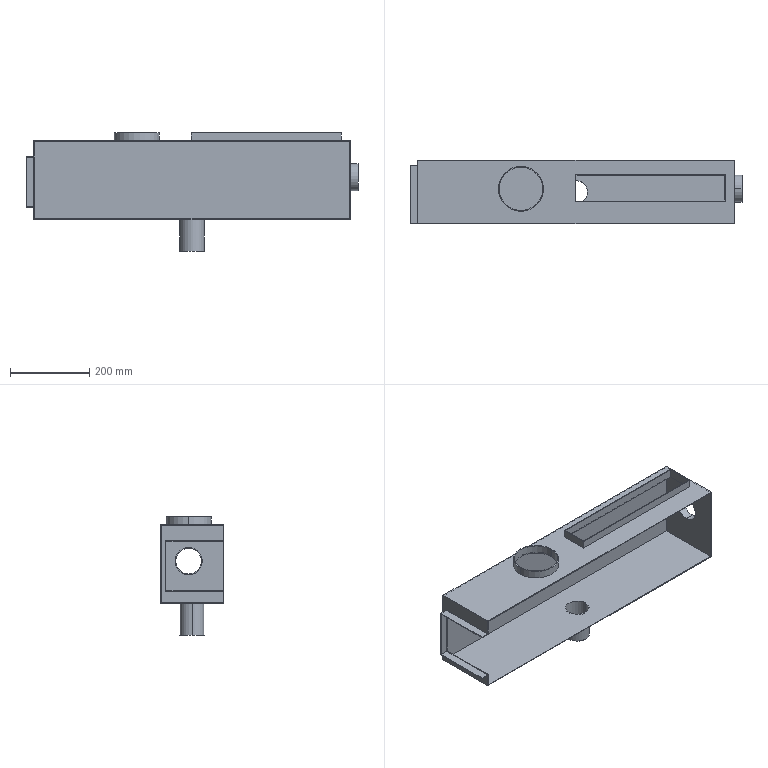Part | NX | features BREP 2 | 2 solids | 48 faces | box 840 x 160 x 300 mm | volume 938258 mm3 | plane 36 | cylinder 12 | commonest cylinder face diameters 58 x2 62 x2 65 x2 69 x2 110 x2 114 x2
STEP:
#1=CARTESIAN_POINT('',(-400.,66.,158.5));
#2=VERTEX_POINT('',#1);
#3=CARTESIAN_POINT('',(-400.,-80.,158.5));
#4=VERTEX_POINT('',#3);
#5=CARTESIAN_POINT('',(-400.,-80.,158.5));
#6=DIRECTION('',(0.,-1.,0.));
#7=VECTOR('',#6,1000.);
#8=LINE('',#5,#7);
#9=EDGE_CURVE('',#2,#4,#8,.T.);
#10=ORIENTED_EDGE('',*,*,#9,.T.);
#11=CARTESIAN_POINT('',(-420.,-80.,158.5));
#12=VERTEX_POINT('',#11);
#13=CARTESIAN_POINT('',(-420.,-80.,158.5));
#14=DIRECTION('',(1.,0.,0.));
#15=VECTOR('',#14,1000.);
#16=LINE('',#13,#15);
#17=EDGE_CURVE('',#12,#4,#16,.T.);
#18=ORIENTED_EDGE('',*,*,#17,.F.);
#19=CARTESIAN_POINT('',(-420.,66.,158.5));
#20=VERTEX_POINT('',#19);
#21=CARTESIAN_POINT('',(-420.,-80.,158.5));
#22=DIRECTION('',(0.,-1.,0.));
#23=VECTOR('',#22,1000.);
#24=LINE('',#21,#23);
#25=EDGE_CURVE('',#20,#12,#24,.T.);
#26=ORIENTED_EDGE('',*,*,#25,.F.);
#27=CARTESIAN_POINT('',(-420.,66.,158.5));
#28=DIRECTION('',(1.,0.,0.));
#29=VECTOR('',#28,1000.);
#30=LINE('',#27,#29);
#31=EDGE_CURVE('',#20,#2,#30,.T.);
#32=ORIENTED_EDGE('',*,*,#31,.T.);
#33=EDGE_LOOP('',(#10,#18,#26,#32));
#34=FACE_BOUND('',#33,.T.);
#35=CARTESIAN_POINT('',(-420.,-80.,158.5));
#36=DIRECTION('',(0.,0.,1.));
#37=DIRECTION('',(1.,0.,0.));
#38=AXIS2_PLACEMENT_3D('',#35,#36,#37);
#39=PLANE('',#38);
#40=ADVANCED_FACE('',(#34),#39,.F.);
#41=CARTESIAN_POINT('',(-400.,-80.,160.5));
#42=VERTEX_POINT('',#41);
#43=CARTESIAN_POINT('',(-400.,-80.,160.5));
#44=DIRECTION('',(0.,0.,-1.));
#45=VECTOR('',#44,1000.);
#46=LINE('',#43,#45);
#47=EDGE_CURVE('',#42,#4,#46,.T.);
#48=ORIENTED_EDGE('',*,*,#47,.F.);
#49=CARTESIAN_POINT('',(-420.,-80.,160.5));
#50=VERTEX_POINT('',#49);
#51=CARTESIAN_POINT('',(-420.,-80.,160.5));
#52=DIRECTION('',(1.,0.,0.));
#53=VECTOR('',#52,1000.);
#54=LINE('',#51,#53);
#55=EDGE_CURVE('',#50,#42,#54,.T.);
#56=ORIENTED_EDGE('',*,*,#55,.F.);
#57=CARTESIAN_POINT('',(-420.,-80.,160.5));
#58=DIRECTION('',(0.,0.,-1.));
#59=VECTOR('',#58,1000.);
#60=LINE('',#57,#59);
#61=EDGE_CURVE('',#50,#12,#60,.T.);
#62=ORIENTED_EDGE('',*,*,#61,.T.);
#63=ORIENTED_EDGE('',*,*,#17,.T.);
#64=EDGE_LOOP('',(#48,#56,#62,#63));
#65=FACE_BOUND('',#64,.T.);
#66=CARTESIAN_POINT('',(-420.,-80.,160.5));
#67=DIRECTION('',(0.,-1.,0.));
#68=DIRECTION('',(0.,0.,-1.));
#69=AXIS2_PLACEMENT_3D('',#66,#67,#68);
#70=PLANE('',#69);
#71=ADVANCED_FACE('',(#65),#70,.T.);
#72=CARTESIAN_POINT('',(-400.,68.,160.5));
#73=VERTEX_POINT('',#72);
#74=CARTESIAN_POINT('',(-400.,-80.,160.5));
#75=DIRECTION('',(0.,-1.,0.));
#76=VECTOR('',#75,1000.);
#77=LINE('',#74,#76);
#78=EDGE_CURVE('',#73,#42,#77,.T.);
#79=ORIENTED_EDGE('',*,*,#78,.F.);
#80=CARTESIAN_POINT('',(-420.,68.,160.5));
#81=VERTEX_POINT('',#80);
#82=CARTESIAN_POINT('',(-420.,68.,160.5));
#83=DIRECTION('',(1.,0.,0.));
#84=VECTOR('',#83,1000.);
#85=LINE('',#82,#84);
#86=EDGE_CURVE('',#81,#73,#85,.T.);
#87=ORIENTED_EDGE('',*,*,#86,.F.);
#88=CARTESIAN_POINT('',(-420.,-80.,160.5));
#89=DIRECTION('',(0.,-1.,0.));
#90=VECTOR('',#89,1000.);
#91=LINE('',#88,#90);
#92=EDGE_CURVE('',#81,#50,#91,.T.);
#93=ORIENTED_EDGE('',*,*,#92,.T.);
#94=ORIENTED_EDGE('',*,*,#55,.T.);
#95=EDGE_LOOP('',(#79,#87,#93,#94));
#96=FACE_BOUND('',#95,.T.);
#97=CARTESIAN_POINT('',(-420.,-80.,160.5));
#98=DIRECTION('',(0.,0.,1.));
#99=DIRECTION('',(1.,0.,0.));
#100=AXIS2_PLACEMENT_3D('',#97,#98,#99);
#101=PLANE('',#100);
#102=ADVANCED_FACE('',(#96),#101,.T.);
#103=CARTESIAN_POINT('',(-400.,68.,31.5));
#104=VERTEX_POINT('',#103);
#105=CARTESIAN_POINT('',(-400.,68.,160.5));
#106=DIRECTION('',(0.,0.,1.));
#107=VECTOR('',#106,1000.);
#108=LINE('',#105,#107);
#109=EDGE_CURVE('',#104,#73,#108,.T.);
#110=ORIENTED_EDGE('',*,*,#109,.F.);
#111=CARTESIAN_POINT('',(-420.,68.,31.5));
#112=VERTEX_POINT('',#111);
#113=CARTESIAN_POINT('',(-420.,68.,31.5));
#114=DIRECTION('',(1.,0.,0.));
#115=VECTOR('',#114,1000.);
#116=LINE('',#113,#115);
#117=EDGE_CURVE('',#112,#104,#116,.T.);
#118=ORIENTED_EDGE('',*,*,#117,.F.);
#119=CARTESIAN_POINT('',(-420.,68.,160.5));
#120=DIRECTION('',(0.,0.,1.));
#121=VECTOR('',#120,1000.);
#122=LINE('',#119,#121);
#123=EDGE_CURVE('',#112,#81,#122,.T.);
#124=ORIENTED_EDGE('',*,*,#123,.T.);
#125=ORIENTED_EDGE('',*,*,#86,.T.);
#126=EDGE_LOOP('',(#110,#118,#124,#125));
#127=FACE_BOUND('',#126,.T.);
#128=CARTESIAN_POINT('',(-420.,68.,160.5));
#129=DIRECTION('',(0.,1.,0.));
#130=DIRECTION('',(1.,0.,0.));
#131=AXIS2_PLACEMENT_3D('',#128,#129,#130);
#132=PLANE('',#131);
#133=ADVANCED_FACE('',(#127),#132,.T.);
#134=CARTESIAN_POINT('',(-400.,-80.,31.5));
#135=VERTEX_POINT('',#134);
#136=CARTESIAN_POINT('',(-400.,-80.,31.5));
#137=DIRECTION('',(0.,1.,0.));
#138=VECTOR('',#137,1000.);
#139=LINE('',#136,#138);
#140=EDGE_CURVE('',#135,#104,#139,.T.);
#141=ORIENTED_EDGE('',*,*,#140,.F.);
#142=CARTESIAN_POINT('',(-420.,-80.,31.5));
#143=VERTEX_POINT('',#142);
#144=CARTESIAN_POINT('',(-420.,-80.,31.5));
#145=DIRECTION('',(1.,0.,0.));
#146=VECTOR('',#145,1000.);
#147=LINE('',#144,#146);
#148=EDGE_CURVE('',#143,#135,#147,.T.);
#149=ORIENTED_EDGE('',*,*,#148,.F.);
#150=CARTESIAN_POINT('',(-420.,-80.,31.5));
#151=DIRECTION('',(0.,1.,0.));
#152=VECTOR('',#151,1000.);
#153=LINE('',#150,#152);
#154=EDGE_CURVE('',#143,#112,#153,.T.);
#155=ORIENTED_EDGE('',*,*,#154,.T.);
#156=ORIENTED_EDGE('',*,*,#117,.T.);
#157=EDGE_LOOP('',(#141,#149,#155,#156));
#158=FACE_BOUND('',#157,.T.);
#159=CARTESIAN_POINT('',(-420.,-80.,31.5));
#160=DIRECTION('',(0.,0.,-1.));
#161=DIRECTION('',(0.,-1.,0.));
#162=AXIS2_PLACEMENT_3D('',#159,#160,#161);
#163=PLANE('',#162);
#164=ADVANCED_FACE('',(#158),#163,.T.);
#165=CARTESIAN_POINT('',(-400.,-80.,33.5));
#166=VERTEX_POINT('',#165);
#167=CARTESIAN_POINT('',(-400.,-80.,33.5));
#168=DIRECTION('',(0.,0.,-1.));
#169=VECTOR('',#168,1000.);
#170=LINE('',#167,#169);
#171=EDGE_CURVE('',#166,#135,#170,.T.);
#172=ORIENTED_EDGE('',*,*,#171,.F.);
#173=CARTESIAN_POINT('',(-420.,-80.,33.5));
#174=VERTEX_POINT('',#173);
#175=CARTESIAN_POINT('',(-420.,-80.,33.5));
#176=DIRECTION('',(1.,0.,0.));
#177=VECTOR('',#176,1000.);
#178=LINE('',#175,#177);
#179=EDGE_CURVE('',#174,#166,#178,.T.);
#180=ORIENTED_EDGE('',*,*,#179,.F.);
#181=CARTESIAN_POINT('',(-420.,-80.,33.5));
#182=DIRECTION('',(0.,0.,-1.));
#183=VECTOR('',#182,1000.);
#184=LINE('',#181,#183);
#185=EDGE_CURVE('',#174,#143,#184,.T.);
#186=ORIENTED_EDGE('',*,*,#185,.T.);
#187=ORIENTED_EDGE('',*,*,#148,.T.);
#188=EDGE_LOOP('',(#172,#180,#186,#187));
#189=FACE_BOUND('',#188,.T.);
#190=CARTESIAN_POINT('',(-420.,-80.,33.5));
#191=DIRECTION('',(0.,-1.,0.));
#192=DIRECTION('',(0.,0.,-1.));
#193=AXIS2_PLACEMENT_3D('',#190,#191,#192);
#194=PLANE('',#193);
#195=ADVANCED_FACE('',(#189),#194,.T.);
#196=CARTESIAN_POINT('',(-400.,66.,33.5));
#197=VERTEX_POINT('',#196);
#198=CARTESIAN_POINT('',(-400.,-80.,33.5));
#199=DIRECTION('',(0.,1.,0.));
#200=VECTOR('',#199,1000.);
#201=LINE('',#198,#200);
#202=EDGE_CURVE('',#166,#197,#201,.T.);
#203=ORIENTED_EDGE('',*,*,#202,.T.);
#204=CARTESIAN_POINT('',(-420.,66.,33.5));
#205=VERTEX_POINT('',#204);
#206=CARTESIAN_POINT('',(-420.,66.,33.5));
#207=DIRECTION('',(1.,0.,0.));
#208=VECTOR('',#207,1000.);
#209=LINE('',#206,#208);
#210=EDGE_CURVE('',#205,#197,#209,.T.);
#211=ORIENTED_EDGE('',*,*,#210,.F.);
#212=CARTESIAN_POINT('',(-420.,-80.,33.5));
#213=DIRECTION('',(0.,1.,0.));
#214=VECTOR('',#213,1000.);
#215=LINE('',#212,#214);
#216=EDGE_CURVE('',#174,#205,#215,.T.);
#217=ORIENTED_EDGE('',*,*,#216,.F.);
#218=ORIENTED_EDGE('',*,*,#179,.T.);
#219=EDGE_LOOP('',(#203,#211,#217,#218));
#220=FACE_BOUND('',#219,.T.);
#221=CARTESIAN_POINT('',(-420.,-80.,33.5));
#222=DIRECTION('',(0.,0.,-1.));
#223=DIRECTION('',(0.,-1.,0.));
#224=AXIS2_PLACEMENT_3D('',#221,#222,#223);
#225=PLANE('',#224);
#226=ADVANCED_FACE('',(#220),#225,.F.);
#227=CARTESIAN_POINT('',(-400.,66.,160.5));
#228=DIRECTION('',(0.,0.,1.));
#229=VECTOR('',#228,1000.);
#230=LINE('',#227,#229);
#231=EDGE_CURVE('',#197,#2,#230,.T.);
#232=ORIENTED_EDGE('',*,*,#231,.T.);
#233=ORIENTED_EDGE('',*,*,#31,.F.);
#234=CARTESIAN_POINT('',(-420.,66.,160.5));
#235=DIRECTION('',(0.,0.,1.));
#236=VECTOR('',#235,1000.);
#237=LINE('',#234,#236);
#238=EDGE_CURVE('',#205,#20,#237,.T.);
#239=ORIENTED_EDGE('',*,*,#238,.F.);
#240=ORIENTED_EDGE('',*,*,#210,.T.);
#241=EDGE_LOOP('',(#232,#233,#239,#240));
#242=FACE_BOUND('',#241,.T.);
#243=CARTESIAN_POINT('',(-420.,66.,160.5));
#244=DIRECTION('',(0.,1.,0.));
#245=DIRECTION('',(1.,0.,0.));
#246=AXIS2_PLACEMENT_3D('',#243,#244,#245);
#247=PLANE('',#246);
#248=ADVANCED_FACE('',(#242),#247,.F.);
#249=ORIENTED_EDGE('',*,*,#25,.T.);
#250=ORIENTED_EDGE('',*,*,#61,.F.);
#251=ORIENTED_EDGE('',*,*,#92,.F.);
#252=ORIENTED_EDGE('',*,*,#123,.F.);
#253=ORIENTED_EDGE('',*,*,#154,.F.);
#254=ORIENTED_EDGE('',*,*,#185,.F.);
#255=ORIENTED_EDGE('',*,*,#216,.T.);
#256=ORIENTED_EDGE('',*,*,#238,.T.);
#257=EDGE_LOOP('',(#249,#250,#251,#252,#253,#254,#255,#256));
#258=FACE_BOUND('',#257,.T.);
#259=CARTESIAN_POINT('',(-420.,0.,0.));
#260=DIRECTION('',(-1.,0.,0.));
#261=DIRECTION('',(0.,0.,1.));
#262=AXIS2_PLACEMENT_3D('',#259,#260,#261);
#263=PLANE('',#262);
#264=ADVANCED_FACE('',(#258),#263,.T.);
#265=ORIENTED_EDGE('',*,*,#9,.F.);
#266=ORIENTED_EDGE('',*,*,#231,.F.);
#267=ORIENTED_EDGE('',*,*,#202,.F.);
#268=ORIENTED_EDGE('',*,*,#171,.T.);
#269=ORIENTED_EDGE('',*,*,#140,.T.);
#270=ORIENTED_EDGE('',*,*,#109,.T.);
#271=ORIENTED_EDGE('',*,*,#78,.T.);
#272=ORIENTED_EDGE('',*,*,#47,.T.);
#273=EDGE_LOOP('',(#265,#266,#267,#268,#269,#270,#271,#272));
#274=FACE_BOUND('',#273,.T.);
#275=CARTESIAN_POINT('',(-400.,0.,0.));
#276=DIRECTION('',(-1.,0.,0.));
#277=DIRECTION('',(0.,0.,1.));
#278=AXIS2_PLACEMENT_3D('',#275,#276,#277);
#279=PLANE('',#278);
#280=ADVANCED_FACE('',(#274),#279,.F.);
#281=CLOSED_SHELL('',(#40,#71,#102,#133,#164,#195,#226,#248,#264,#280));
#282=MANIFOLD_SOLID_BREP('',#281);
#283=CARTESIAN_POINT('',(-31.,0.,-80.));
#284=VERTEX_POINT('',#283);
#285=CARTESIAN_POINT('',(31.,0.,-80.));
#286=VERTEX_POINT('',#285);
#287=CARTESIAN_POINT('',(0.,0.,-80.));
#288=DIRECTION('',(0.,0.,-1.));
#289=DIRECTION('',(-1.,0.,0.));
#290=AXIS2_PLACEMENT_3D('',#287,#288,#289);
#291=CIRCLE('',#290,31.);
#292=EDGE_CURVE('',#284,#286,#291,.T.);
#293=ORIENTED_EDGE('',*,*,#292,.F.);
#294=CARTESIAN_POINT('',(-31.,0.,0.));
#295=VERTEX_POINT('',#294);
#296=CARTESIAN_POINT('',(-31.,0.,-80.));
#297=DIRECTION('',(0.,0.,1.));
#298=VECTOR('',#297,1000.);
#299=LINE('',#296,#298);
#300=EDGE_CURVE('',#295,#284,#299,.F.);
#301=ORIENTED_EDGE('',*,*,#300,.F.);
#302=CARTESIAN_POINT('',(31.,0.,0.));
#303=VERTEX_POINT('',#302);
#304=CARTESIAN_POINT('',(0.,0.,0.));
#305=DIRECTION('',(0.,0.,-1.));
#306=DIRECTION('',(1.,0.,0.));
#307=AXIS2_PLACEMENT_3D('',#304,#305,#306);
#308=CIRCLE('',#307,31.);
#309=EDGE_CURVE('',#295,#303,#308,.T.);
#310=ORIENTED_EDGE('',*,*,#309,.T.);
#311=CARTESIAN_POINT('',(31.,0.,-80.));
#312=DIRECTION('',(0.,0.,1.));
#313=VECTOR('',#312,1000.);
#314=LINE('',#311,#313);
#315=EDGE_CURVE('',#303,#286,#314,.F.);
#316=ORIENTED_EDGE('',*,*,#315,.T.);
#317=EDGE_LOOP('',(#293,#301,#310,#316));
#318=FACE_BOUND('',#317,.T.);
#319=CARTESIAN_POINT('',(0.,0.,-80.));
#320=DIRECTION('',(0.,0.,1.));
#321=DIRECTION('',(1.,0.,0.));
#322=AXIS2_PLACEMENT_3D('',#319,#320,#321);
#323=CYLINDRICAL_SURFACE('',#322,31.);
#324=ADVANCED_FACE('',(#318),#323,.T.);
#325=CARTESIAN_POINT('',(-29.,0.,2.));
#326=VERTEX_POINT('',#325);
#327=CARTESIAN_POINT('',(29.,0.,2.));
#328=VERTEX_POINT('',#327);
#329=CARTESIAN_POINT('',(0.,0.,2.));
#330=DIRECTION('',(0.,0.,1.));
#331=DIRECTION('',(1.,0.,0.));
#332=AXIS2_PLACEMENT_3D('',#329,#330,#331);
#333=CIRCLE('',#332,29.);
#334=EDGE_CURVE('',#326,#328,#333,.T.);
#335=ORIENTED_EDGE('',*,*,#334,.T.);
#336=CARTESIAN_POINT('',(29.,0.,-80.));
#337=VERTEX_POINT('',#336);
#338=CARTESIAN_POINT('',(29.,0.,20.));
#339=DIRECTION('',(0.,0.,-1.));
#340=VECTOR('',#339,1000.);
#341=LINE('',#338,#340);
#342=EDGE_CURVE('',#328,#337,#341,.T.);
#343=ORIENTED_EDGE('',*,*,#342,.T.);
#344=CARTESIAN_POINT('',(-29.,0.,-80.));
#345=VERTEX_POINT('',#344);
#346=CARTESIAN_POINT('',(0.,0.,-80.));
#347=DIRECTION('',(0.,0.,-1.));
#348=DIRECTION('',(-1.,0.,0.));
#349=AXIS2_PLACEMENT_3D('',#346,#347,#348);
#350=CIRCLE('',#349,29.);
#351=EDGE_CURVE('',#337,#345,#350,.T.);
#352=ORIENTED_EDGE('',*,*,#351,.T.);
#353=CARTESIAN_POINT('',(-29.,0.,20.));
#354=DIRECTION('',(0.,0.,-1.));
#355=VECTOR('',#354,1000.);
#356=LINE('',#353,#355);
#357=EDGE_CURVE('',#326,#345,#356,.T.);
#358=ORIENTED_EDGE('',*,*,#357,.F.);
#359=EDGE_LOOP('',(#335,#343,#352,#358));
#360=FACE_BOUND('',#359,.T.);
#361=CARTESIAN_POINT('',(0.,0.,20.));
#362=DIRECTION('',(0.,0.,-1.));
#363=DIRECTION('',(-1.,0.,0.));
#364=AXIS2_PLACEMENT_3D('',#361,#362,#363);
#365=CYLINDRICAL_SURFACE('',#364,29.);
#366=ADVANCED_FACE('',(#360),#365,.F.);
#367=CARTESIAN_POINT('',(420.,8.35,140.05));
#368=VERTEX_POINT('',#367);
#369=CARTESIAN_POINT('',(420.,8.35,75.05));
#370=VERTEX_POINT('',#369);
#371=CARTESIAN_POINT('',(420.,8.35,107.55));
#372=DIRECTION('',(1.,0.,0.));
#373=DIRECTION('',(0.,0.,-1.));
#374=AXIS2_PLACEMENT_3D('',#371,#372,#373);
#375=CIRCLE('',#374,32.5);
#376=EDGE_CURVE('',#368,#370,#375,.T.);
#377=ORIENTED_EDGE('',*,*,#376,.T.);
#378=CARTESIAN_POINT('',(398.,8.35,75.05));
#379=VERTEX_POINT('',#378);
#380=CARTESIAN_POINT('',(420.,8.35,75.05));
#381=DIRECTION('',(-1.,0.,0.));
#382=VECTOR('',#381,1000.);
#383=LINE('',#380,#382);
#384=EDGE_CURVE('',#379,#370,#383,.F.);
#385=ORIENTED_EDGE('',*,*,#384,.F.);
#386=CARTESIAN_POINT('',(398.,8.35,140.05));
#387=VERTEX_POINT('',#386);
#388=CARTESIAN_POINT('',(398.,8.35,107.55));
#389=DIRECTION('',(-1.,0.,0.));
#390=DIRECTION('',(0.,0.,1.));
#391=AXIS2_PLACEMENT_3D('',#388,#389,#390);
#392=CIRCLE('',#391,32.5);
#393=EDGE_CURVE('',#379,#387,#392,.T.);
#394=ORIENTED_EDGE('',*,*,#393,.T.);
#395=CARTESIAN_POINT('',(420.,8.35,140.05));
#396=DIRECTION('',(-1.,0.,0.));
#397=VECTOR('',#396,1000.);
#398=LINE('',#395,#397);
#399=EDGE_CURVE('',#387,#368,#398,.F.);
#400=ORIENTED_EDGE('',*,*,#399,.T.);
#401=EDGE_LOOP('',(#377,#385,#394,#400));
#402=FACE_BOUND('',#401,.T.);
#403=CARTESIAN_POINT('',(420.,8.35,107.55));
#404=DIRECTION('',(-1.,0.,0.));
#405=DIRECTION('',(0.,0.,1.));
#406=AXIS2_PLACEMENT_3D('',#403,#404,#405);
#407=CYLINDRICAL_SURFACE('',#406,32.5);
#408=ADVANCED_FACE('',(#402),#407,.F.);
#409=CARTESIAN_POINT('',(420.,8.35,73.05));
#410=VERTEX_POINT('',#409);
#411=CARTESIAN_POINT('',(420.,8.35,142.05));
#412=VERTEX_POINT('',#411);
#413=CARTESIAN_POINT('',(420.,8.35,107.55));
#414=DIRECTION('',(1.,0.,0.));
#415=DIRECTION('',(0.,0.,-1.));
#416=AXIS2_PLACEMENT_3D('',#413,#414,#415);
#417=CIRCLE('',#416,34.5);
#418=EDGE_CURVE('',#410,#412,#417,.T.);
#419=ORIENTED_EDGE('',*,*,#418,.F.);
#420=CARTESIAN_POINT('',(400.,8.35,73.05));
#421=VERTEX_POINT('',#420);
#422=CARTESIAN_POINT('',(420.,8.35,73.05));
#423=DIRECTION('',(-1.,0.,0.));
#424=VECTOR('',#423,1000.);
#425=LINE('',#422,#424);
#426=EDGE_CURVE('',#421,#410,#425,.F.);
#427=ORIENTED_EDGE('',*,*,#426,.F.);
#428=CARTESIAN_POINT('',(400.,8.35,142.05));
#429=VERTEX_POINT('',#428);
#430=CARTESIAN_POINT('',(400.,8.35,107.55));
#431=DIRECTION('',(1.,0.,0.));
#432=DIRECTION('',(0.,0.,1.));
#433=AXIS2_PLACEMENT_3D('',#430,#431,#432);
#434=CIRCLE('',#433,34.5);
#435=EDGE_CURVE('',#421,#429,#434,.T.);
#436=ORIENTED_EDGE('',*,*,#435,.T.);
#437=CARTESIAN_POINT('',(420.,8.35,142.05));
#438=DIRECTION('',(-1.,0.,0.));
#439=VECTOR('',#438,1000.);
#440=LINE('',#437,#439);
#441=EDGE_CURVE('',#429,#412,#440,.F.);
#442=ORIENTED_EDGE('',*,*,#441,.T.);
#443=EDGE_LOOP('',(#419,#427,#436,#442));
#444=FACE_BOUND('',#443,.T.);
#445=CARTESIAN_POINT('',(420.,8.35,107.55));
#446=DIRECTION('',(-1.,0.,0.));
#447=DIRECTION('',(0.,0.,1.));
#448=AXIS2_PLACEMENT_3D('',#445,#446,#447);
#449=CYLINDRICAL_SURFACE('',#448,34.5);
#450=ADVANCED_FACE('',(#444),#449,.T.);
#451=CARTESIAN_POINT('',(-82.25,8.,220.));
#452=VERTEX_POINT('',#451);
#453=CARTESIAN_POINT('',(-196.25,8.,220.));
#454=VERTEX_POINT('',#453);
#455=CARTESIAN_POINT('',(-139.25,8.,220.));
#456=DIRECTION('',(0.,0.,1.));
#457=DIRECTION('',(1.,0.,0.));
#458=AXIS2_PLACEMENT_3D('',#455,#456,#457);
#459=CIRCLE('',#458,57.);
#460=EDGE_CURVE('',#452,#454,#459,.T.);
#461=ORIENTED_EDGE('',*,*,#460,.F.);
#462=CARTESIAN_POINT('',(-82.25,8.,200.));
#463=VERTEX_POINT('',#462);
#464=CARTESIAN_POINT('',(-82.25,8.,220.));
#465=DIRECTION('',(0.,0.,-1.));
#466=VECTOR('',#465,1000.);
#467=LINE('',#464,#466);
#468=EDGE_CURVE('',#452,#463,#467,.T.);
#469=ORIENTED_EDGE('',*,*,#468,.T.);
#470=CARTESIAN_POINT('',(-196.25,8.,200.));
#471=VERTEX_POINT('',#470);
#472=CARTESIAN_POINT('',(-139.25,8.,200.));
#473=DIRECTION('',(0.,0.,1.));
#474=DIRECTION('',(1.,0.,0.));
#475=AXIS2_PLACEMENT_3D('',#472,#473,#474);
#476=CIRCLE('',#475,57.);
#477=EDGE_CURVE('',#463,#471,#476,.T.);
#478=ORIENTED_EDGE('',*,*,#477,.T.);
#479=CARTESIAN_POINT('',(-196.25,8.,220.));
#480=DIRECTION('',(0.,0.,-1.));
#481=VECTOR('',#480,1000.);
#482=LINE('',#479,#481);
#483=EDGE_CURVE('',#454,#471,#482,.T.);
#484=ORIENTED_EDGE('',*,*,#483,.F.);
#485=EDGE_LOOP('',(#461,#469,#478,#484));
#486=FACE_BOUND('',#485,.T.);
#487=CARTESIAN_POINT('',(-139.25,8.,220.));
#488=DIRECTION('',(0.,0.,-1.));
#489=DIRECTION('',(-1.,0.,0.));
#490=AXIS2_PLACEMENT_3D('',#487,#488,#489);
#491=CYLINDRICAL_SURFACE('',#490,57.);
#492=ADVANCED_FACE('',(#486),#491,.T.);
#493=CARTESIAN_POINT('',(-194.25,8.,198.));
#494=VERTEX_POINT('',#493);
#495=CARTESIAN_POINT('',(-84.25,8.,198.));
#496=VERTEX_POINT('',#495);
#497=CARTESIAN_POINT('',(-139.25,8.,198.));
#498=DIRECTION('',(0.,0.,1.));
#499=DIRECTION('',(1.,0.,0.));
#500=AXIS2_PLACEMENT_3D('',#497,#498,#499);
#501=CIRCLE('',#500,55.);
#502=EDGE_CURVE('',#494,#496,#501,.T.);
#503=ORIENTED_EDGE('',*,*,#502,.F.);
#504=CARTESIAN_POINT('',(-194.25,8.,220.));
#505=VERTEX_POINT('',#504);
#506=CARTESIAN_POINT('',(-194.25,8.,185.));
#507=DIRECTION('',(0.,0.,1.));
#508=VECTOR('',#507,1000.);
#509=LINE('',#506,#508);
#510=EDGE_CURVE('',#505,#494,#509,.F.);
#511=ORIENTED_EDGE('',*,*,#510,.F.);
#512=CARTESIAN_POINT('',(-84.25,8.,220.));
#513=VERTEX_POINT('',#512);
#514=CARTESIAN_POINT('',(-139.25,8.,220.));
#515=DIRECTION('',(0.,0.,1.));
#516=DIRECTION('',(1.,0.,0.));
#517=AXIS2_PLACEMENT_3D('',#514,#515,#516);
#518=CIRCLE('',#517,55.);
#519=EDGE_CURVE('',#505,#513,#518,.T.);
#520=ORIENTED_EDGE('',*,*,#519,.T.);
#521=CARTESIAN_POINT('',(-84.25,8.,185.));
#522=DIRECTION('',(0.,0.,1.));
#523=VECTOR('',#522,1000.);
#524=LINE('',#521,#523);
#525=EDGE_CURVE('',#513,#496,#524,.F.);
#526=ORIENTED_EDGE('',*,*,#525,.T.);
#527=EDGE_LOOP('',(#503,#511,#520,#526));
#528=FACE_BOUND('',#527,.T.);
#529=CARTESIAN_POINT('',(-139.25,8.,185.));
#530=DIRECTION('',(0.,0.,1.));
#531=DIRECTION('',(1.,0.,0.));
#532=AXIS2_PLACEMENT_3D('',#529,#530,#531);
#533=CYLINDRICAL_SURFACE('',#532,55.);
#534=ADVANCED_FACE('',(#528),#533,.F.);
#535=CARTESIAN_POINT('',(-400.,80.,200.));
#536=VERTEX_POINT('',#535);
#537=CARTESIAN_POINT('',(-400.,-80.,200.));
#538=VERTEX_POINT('',#537);
#539=CARTESIAN_POINT('',(-400.,-80.,200.));
#540=DIRECTION('',(0.,-1.,0.));
#541=VECTOR('',#540,1000.);
#542=LINE('',#539,#541);
#543=EDGE_CURVE('',#536,#538,#542,.T.);
#544=ORIENTED_EDGE('',*,*,#543,.T.);
#545=CARTESIAN_POINT('',(400.,-80.,200.));
#546=VERTEX_POINT('',#545);
#547=CARTESIAN_POINT('',(400.,-80.,200.));
#548=DIRECTION('',(1.,0.,0.));
#549=VECTOR('',#548,1000.);
#550=LINE('',#547,#549);
#551=EDGE_CURVE('',#538,#546,#550,.T.);
#552=ORIENTED_EDGE('',*,*,#551,.T.);
#553=CARTESIAN_POINT('',(400.,80.,200.));
#554=VERTEX_POINT('',#553);
#555=CARTESIAN_POINT('',(400.,-80.,200.));
#556=DIRECTION('',(0.,1.,0.));
#557=VECTOR('',#556,1000.);
#558=LINE('',#555,#557);
#559=EDGE_CURVE('',#546,#554,#558,.T.);
#560=ORIENTED_EDGE('',*,*,#559,.T.);
#561=CARTESIAN_POINT('',(400.,80.,200.));
#562=DIRECTION('',(-1.,0.,0.));
#563=VECTOR('',#562,1000.);
#564=LINE('',#561,#563);
#565=EDGE_CURVE('',#554,#536,#564,.T.);
#566=ORIENTED_EDGE('',*,*,#565,.T.);
#567=EDGE_LOOP('',(#544,#552,#560,#566));
#568=FACE_BOUND('',#567,.T.);
#569=CARTESIAN_POINT('',(-139.25,8.,200.));
#570=DIRECTION('',(0.,0.,1.));
#571=DIRECTION('',(1.,0.,0.));
#572=AXIS2_PLACEMENT_3D('',#569,#570,#571);
#573=CIRCLE('',#572,57.);
#574=EDGE_CURVE('',#471,#463,#573,.T.);
#575=ORIENTED_EDGE('',*,*,#574,.F.);
#576=ORIENTED_EDGE('',*,*,#477,.F.);
#577=EDGE_LOOP('',(#575,#576));
#578=FACE_BOUND('',#577,.T.);
#579=CARTESIAN_POINT('',(378.,-25.,200.));
#580=VERTEX_POINT('',#579);
#581=CARTESIAN_POINT('',(378.,44.,200.));
#582=VERTEX_POINT('',#581);
#583=CARTESIAN_POINT('',(378.,-25.,200.));
#584=DIRECTION('',(0.,1.,0.));
#585=VECTOR('',#584,1000.);
#586=LINE('',#583,#585);
#587=EDGE_CURVE('',#580,#582,#586,.T.);
#588=ORIENTED_EDGE('',*,*,#587,.F.);
#589=CARTESIAN_POINT('',(-2.,-25.,200.));
#590=VERTEX_POINT('',#589);
#591=CARTESIAN_POINT('',(378.,-25.,200.));
#592=DIRECTION('',(1.,0.,0.));
#593=VECTOR('',#592,1000.);
#594=LINE('',#591,#593);
#595=EDGE_CURVE('',#590,#580,#594,.T.);
#596=ORIENTED_EDGE('',*,*,#595,.F.);
#597=CARTESIAN_POINT('',(-2.,44.,200.));
#598=VERTEX_POINT('',#597);
#599=CARTESIAN_POINT('',(-2.,-25.,200.));
#600=DIRECTION('',(0.,-1.,0.));
#601=VECTOR('',#600,1000.);
#602=LINE('',#599,#601);
#603=EDGE_CURVE('',#598,#590,#602,.T.);
#604=ORIENTED_EDGE('',*,*,#603,.F.);
#605=CARTESIAN_POINT('',(378.,44.,200.));
#606=DIRECTION('',(-1.,0.,0.));
#607=VECTOR('',#606,1000.);
#608=LINE('',#605,#607);
#609=EDGE_CURVE('',#582,#598,#608,.T.);
#610=ORIENTED_EDGE('',*,*,#609,.F.);
#611=EDGE_LOOP('',(#588,#596,#604,#610));
#612=FACE_BOUND('',#611,.T.);
#613=CARTESIAN_POINT('',(0.,0.,200.));
#614=DIRECTION('',(0.,0.,1.));
#615=DIRECTION('',(1.,0.,0.));
#616=AXIS2_PLACEMENT_3D('',#613,#614,#615);
#617=PLANE('',#616);
#618=ADVANCED_FACE('',(#568,#578,#612),#617,.T.);
#619=CARTESIAN_POINT('',(-400.,80.,0.));
#620=VERTEX_POINT('',#619);
#621=CARTESIAN_POINT('',(-400.,-80.,0.));
#622=VERTEX_POINT('',#621);
#623=CARTESIAN_POINT('',(-400.,-80.,0.));
#624=DIRECTION('',(0.,-1.,0.));
#625=VECTOR('',#624,1000.);
#626=LINE('',#623,#625);
#627=EDGE_CURVE('',#620,#622,#626,.T.);
#628=ORIENTED_EDGE('',*,*,#627,.F.);
#629=CARTESIAN_POINT('',(400.,80.,0.));
#630=VERTEX_POINT('',#629);
#631=CARTESIAN_POINT('',(400.,80.,0.));
#632=DIRECTION('',(-1.,0.,0.));
#633=VECTOR('',#632,1000.);
#634=LINE('',#631,#633);
#635=EDGE_CURVE('',#630,#620,#634,.T.);
#636=ORIENTED_EDGE('',*,*,#635,.F.);
#637=CARTESIAN_POINT('',(400.,-80.,0.));
#638=VERTEX_POINT('',#637);
#639=CARTESIAN_POINT('',(400.,-80.,0.));
#640=DIRECTION('',(0.,1.,0.));
#641=VECTOR('',#640,1000.);
#642=LINE('',#639,#641);
#643=EDGE_CURVE('',#638,#630,#642,.T.);
#644=ORIENTED_EDGE('',*,*,#643,.F.);
#645=CARTESIAN_POINT('',(400.,-80.,0.));
#646=DIRECTION('',(1.,0.,0.));
#647=VECTOR('',#646,1000.);
#648=LINE('',#645,#647);
#649=EDGE_CURVE('',#622,#638,#648,.T.);
#650=ORIENTED_EDGE('',*,*,#649,.F.);
#651=EDGE_LOOP('',(#628,#636,#644,#650));
#652=FACE_BOUND('',#651,.T.);
#653=CARTESIAN_POINT('',(0.,0.,0.));
#654=DIRECTION('',(0.,0.,-1.));
#655=DIRECTION('',(1.,0.,0.));
#656=AXIS2_PLACEMENT_3D('',#653,#654,#655);
#657=CIRCLE('',#656,31.);
#658=EDGE_CURVE('',#303,#295,#657,.T.);
#659=ORIENTED_EDGE('',*,*,#658,.F.);
#660=ORIENTED_EDGE('',*,*,#309,.F.);
#661=EDGE_LOOP('',(#659,#660));
#662=FACE_BOUND('',#661,.T.);
#663=CARTESIAN_POINT('',(0.,0.,0.));
#664=DIRECTION('',(0.,0.,1.));
#665=DIRECTION('',(1.,0.,0.));
#666=AXIS2_PLACEMENT_3D('',#663,#664,#665);
#667=PLANE('',#666);
#668=ADVANCED_FACE('',(#652,#662),#667,.F.);
#669=CARTESIAN_POINT('',(-398.,-80.,33.5));
#670=VERTEX_POINT('',#669);
#671=CARTESIAN_POINT('',(-398.,-80.,2.));
#672=VERTEX_POINT('',#671);
#673=CARTESIAN_POINT('',(-398.,-80.,200.));
#674=DIRECTION('',(0.,0.,-1.));
#675=VECTOR('',#674,1000.);
#676=LINE('',#673,#675);
#677=EDGE_CURVE('',#670,#672,#676,.T.);
#678=ORIENTED_EDGE('',*,*,#677,.F.);
#679=CARTESIAN_POINT('',(-400.,-80.,33.5));
#680=VERTEX_POINT('',#679);
#681=CARTESIAN_POINT('',(400.,-80.,33.5));
#682=DIRECTION('',(-1.,0.,0.));
#683=VECTOR('',#682,1000.);
#684=LINE('',#681,#683);
#685=EDGE_CURVE('',#670,#680,#684,.T.);
#686=ORIENTED_EDGE('',*,*,#685,.T.);
#687=CARTESIAN_POINT('',(-400.,-80.,200.));
#688=DIRECTION('',(0.,0.,-1.));
#689=VECTOR('',#688,1000.);
#690=LINE('',#687,#689);
#691=EDGE_CURVE('',#680,#622,#690,.T.);
#692=ORIENTED_EDGE('',*,*,#691,.T.);
#693=ORIENTED_EDGE('',*,*,#649,.T.);
#694=CARTESIAN_POINT('',(400.,-80.,200.));
#695=DIRECTION('',(0.,0.,-1.));
#696=VECTOR('',#695,1000.);
#697=LINE('',#694,#696);
#698=EDGE_CURVE('',#546,#638,#697,.T.);
#699=ORIENTED_EDGE('',*,*,#698,.F.);
#700=ORIENTED_EDGE('',*,*,#551,.F.);
#701=CARTESIAN_POINT('',(-400.,-80.,158.5));
#702=VERTEX_POINT('',#701);
#703=CARTESIAN_POINT('',(-400.,-80.,200.));
#704=DIRECTION('',(0.,0.,-1.));
#705=VECTOR('',#704,1000.);
#706=LINE('',#703,#705);
#707=EDGE_CURVE('',#538,#702,#706,.T.);
#708=ORIENTED_EDGE('',*,*,#707,.T.);
#709=CARTESIAN_POINT('',(-398.,-80.,158.5));
#710=VERTEX_POINT('',#709);
#711=CARTESIAN_POINT('',(400.,-80.,158.5));
#712=DIRECTION('',(1.,0.,0.));
#713=VECTOR('',#712,1000.);
#714=LINE('',#711,#713);
#715=EDGE_CURVE('',#702,#710,#714,.T.);
#716=ORIENTED_EDGE('',*,*,#715,.T.);
#717=CARTESIAN_POINT('',(-398.,-80.,198.));
#718=VERTEX_POINT('',#717);
#719=CARTESIAN_POINT('',(-398.,-80.,200.));
#720=DIRECTION('',(0.,0.,-1.));
#721=VECTOR('',#720,1000.);
#722=LINE('',#719,#721);
#723=EDGE_CURVE('',#718,#710,#722,.T.);
#724=ORIENTED_EDGE('',*,*,#723,.F.);
#725=CARTESIAN_POINT('',(398.,-80.,198.));
#726=VERTEX_POINT('',#725);
#727=CARTESIAN_POINT('',(400.,-80.,198.));
#728=DIRECTION('',(1.,0.,0.));
#729=VECTOR('',#728,1000.);
#730=LINE('',#727,#729);
#731=EDGE_CURVE('',#718,#726,#730,.T.);
#732=ORIENTED_EDGE('',*,*,#731,.T.);
#733=CARTESIAN_POINT('',(398.,-80.,2.));
#734=VERTEX_POINT('',#733);
#735=CARTESIAN_POINT('',(398.,-80.,200.));
#736=DIRECTION('',(0.,0.,-1.));
#737=VECTOR('',#736,1000.);
#738=LINE('',#735,#737);
#739=EDGE_CURVE('',#726,#734,#738,.T.);
#740=ORIENTED_EDGE('',*,*,#739,.T.);
#741=CARTESIAN_POINT('',(400.,-80.,2.));
#742=DIRECTION('',(1.,0.,0.));
#743=VECTOR('',#742,1000.);
#744=LINE('',#741,#743);
#745=EDGE_CURVE('',#672,#734,#744,.T.);
#746=ORIENTED_EDGE('',*,*,#745,.F.);
#747=EDGE_LOOP('',(#678,#686,#692,#693,#699,#700,#708,#716,#724,#732,#740,#746));
#748=FACE_BOUND('',#747,.T.);
#749=CARTESIAN_POINT('',(400.,-80.,200.));
#750=DIRECTION('',(0.,1.,0.));
#751=DIRECTION('',(1.,0.,0.));
#752=AXIS2_PLACEMENT_3D('',#749,#750,#751);
#753=PLANE('',#752);
#754=ADVANCED_FACE('',(#748),#753,.F.);
#755=CARTESIAN_POINT('',(-400.,66.,158.5));
#756=VERTEX_POINT('',#755);
#757=CARTESIAN_POINT('',(-400.,66.,33.5));
#758=VERTEX_POINT('',#757);
#759=CARTESIAN_POINT('',(-400.,66.,113.5));
#760=DIRECTION('',(0.,0.,-1.));
#761=VECTOR('',#760,1000.);
#762=LINE('',#759,#761);
#763=EDGE_CURVE('',#756,#758,#762,.T.);
#764=ORIENTED_EDGE('',*,*,#763,.F.);
#765=CARTESIAN_POINT('',(-400.,21.,158.5));
#766=DIRECTION('',(0.,1.,0.));
#767=VECTOR('',#766,1000.);
#768=LINE('',#765,#767);
#769=EDGE_CURVE('',#702,#756,#768,.T.);
#770=ORIENTED_EDGE('',*,*,#769,.F.);
#771=ORIENTED_EDGE('',*,*,#707,.F.);
#772=ORIENTED_EDGE('',*,*,#543,.F.);
#773=CARTESIAN_POINT('',(-400.,80.,200.));
#774=DIRECTION('',(0.,0.,-1.));
#775=VECTOR('',#774,1000.);
#776=LINE('',#773,#775);
#777=EDGE_CURVE('',#536,#620,#776,.T.);
#778=ORIENTED_EDGE('',*,*,#777,.T.);
#779=ORIENTED_EDGE('',*,*,#627,.T.);
#780=ORIENTED_EDGE('',*,*,#691,.F.);
#781=CARTESIAN_POINT('',(-400.,66.,33.5));
#782=DIRECTION('',(0.,-1.,0.));
#783=VECTOR('',#782,1000.);
#784=LINE('',#781,#783);
#785=EDGE_CURVE('',#758,#680,#784,.T.);
#786=ORIENTED_EDGE('',*,*,#785,.F.);
#787=EDGE_LOOP('',(#764,#770,#771,#772,#778,#779,#780,#786));
#788=FACE_BOUND('',#787,.T.);
#789=CARTESIAN_POINT('',(-400.,-80.,200.));
#790=DIRECTION('',(1.,0.,0.));
#791=DIRECTION('',(0.,1.,0.));
#792=AXIS2_PLACEMENT_3D('',#789,#790,#791);
#793=PLANE('',#792);
#794=ADVANCED_FACE('',(#788),#793,.F.);
#795=ORIENTED_EDGE('',*,*,#643,.T.);
#796=CARTESIAN_POINT('',(400.,80.,200.));
#797=DIRECTION('',(0.,0.,-1.));
#798=VECTOR('',#797,1000.);
#799=LINE('',#796,#798);
#800=EDGE_CURVE('',#554,#630,#799,.T.);
#801=ORIENTED_EDGE('',*,*,#800,.F.);
#802=ORIENTED_EDGE('',*,*,#559,.F.);
#803=ORIENTED_EDGE('',*,*,#698,.T.);
#804=EDGE_LOOP('',(#795,#801,#802,#803));
#805=FACE_BOUND('',#804,.T.);
#806=CARTESIAN_POINT('',(400.,8.35,107.55));
#807=DIRECTION('',(1.,0.,0.));
#808=DIRECTION('',(0.,0.,1.));
#809=AXIS2_PLACEMENT_3D('',#806,#807,#808);
#810=CIRCLE('',#809,34.5);
#811=EDGE_CURVE('',#429,#421,#810,.T.);
#812=ORIENTED_EDGE('',*,*,#811,.F.);
#813=ORIENTED_EDGE('',*,*,#435,.F.);
#814=EDGE_LOOP('',(#812,#813));
#815=FACE_BOUND('',#814,.T.);
#816=CARTESIAN_POINT('',(400.,-80.,200.));
#817=DIRECTION('',(-1.,0.,0.));
#818=DIRECTION('',(0.,0.,1.));
#819=AXIS2_PLACEMENT_3D('',#816,#817,#818);
#820=PLANE('',#819);
#821=ADVANCED_FACE('',(#805,#815),#820,.F.);
#822=ORIENTED_EDGE('',*,*,#635,.T.);
#823=ORIENTED_EDGE('',*,*,#777,.F.);
#824=ORIENTED_EDGE('',*,*,#565,.F.);
#825=ORIENTED_EDGE('',*,*,#800,.T.);
#826=EDGE_LOOP('',(#822,#823,#824,#825));
#827=FACE_BOUND('',#826,.T.);
#828=CARTESIAN_POINT('',(400.,80.,200.));
#829=DIRECTION('',(0.,-1.,0.));
#830=DIRECTION('',(0.,0.,-1.));
#831=AXIS2_PLACEMENT_3D('',#828,#829,#830);
#832=PLANE('',#831);
#833=ADVANCED_FACE('',(#827),#832,.F.);
#834=CARTESIAN_POINT('',(-398.,66.,158.5));
#835=VERTEX_POINT('',#834);
#836=CARTESIAN_POINT('',(-398.,-80.,158.5));
#837=DIRECTION('',(0.,-1.,0.));
#838=VECTOR('',#837,1000.);
#839=LINE('',#836,#838);
#840=EDGE_CURVE('',#835,#710,#839,.T.);
#841=ORIENTED_EDGE('',*,*,#840,.F.);
#842=CARTESIAN_POINT('',(-398.,66.,33.5));
#843=VERTEX_POINT('',#842);
#844=CARTESIAN_POINT('',(-398.,66.,200.));
#845=DIRECTION('',(0.,0.,1.));
#846=VECTOR('',#845,1000.);
#847=LINE('',#844,#846);
#848=EDGE_CURVE('',#843,#835,#847,.T.);
#849=ORIENTED_EDGE('',*,*,#848,.F.);
#850=CARTESIAN_POINT('',(-398.,-80.,33.5));
#851=DIRECTION('',(0.,1.,0.));
#852=VECTOR('',#851,1000.);
#853=LINE('',#850,#852);
#854=EDGE_CURVE('',#670,#843,#853,.T.);
#855=ORIENTED_EDGE('',*,*,#854,.F.);
#856=ORIENTED_EDGE('',*,*,#677,.T.);
#857=CARTESIAN_POINT('',(-398.,78.,2.));
#858=VERTEX_POINT('',#857);
#859=CARTESIAN_POINT('',(-398.,-80.,2.));
#860=DIRECTION('',(0.,-1.,0.));
#861=VECTOR('',#860,1000.);
#862=LINE('',#859,#861);
#863=EDGE_CURVE('',#858,#672,#862,.T.);
#864=ORIENTED_EDGE('',*,*,#863,.F.);
#865=CARTESIAN_POINT('',(-398.,78.,198.));
#866=VERTEX_POINT('',#865);
#867=CARTESIAN_POINT('',(-398.,78.,200.));
#868=DIRECTION('',(0.,0.,-1.));
#869=VECTOR('',#868,1000.);
#870=LINE('',#867,#869);
#871=EDGE_CURVE('',#866,#858,#870,.T.);
#872=ORIENTED_EDGE('',*,*,#871,.F.);
#873=CARTESIAN_POINT('',(-398.,-80.,198.));
#874=DIRECTION('',(0.,-1.,0.));
#875=VECTOR('',#874,1000.);
#876=LINE('',#873,#875);
#877=EDGE_CURVE('',#866,#718,#876,.T.);
#878=ORIENTED_EDGE('',*,*,#877,.T.);
#879=ORIENTED_EDGE('',*,*,#723,.T.);
#880=EDGE_LOOP('',(#841,#849,#855,#856,#864,#872,#878,#879));
#881=FACE_BOUND('',#880,.T.);
#882=CARTESIAN_POINT('',(-398.,-80.,200.));
#883=DIRECTION('',(1.,0.,0.));
#884=DIRECTION('',(0.,1.,0.));
#885=AXIS2_PLACEMENT_3D('',#882,#883,#884);
#886=PLANE('',#885);
#887=ADVANCED_FACE('',(#881),#886,.T.);
#888=CARTESIAN_POINT('',(398.,78.,2.));
#889=VERTEX_POINT('',#888);
#890=CARTESIAN_POINT('',(398.,-80.,2.));
#891=DIRECTION('',(0.,1.,0.));
#892=VECTOR('',#891,1000.);
#893=LINE('',#890,#892);
#894=EDGE_CURVE('',#734,#889,#893,.T.);
#895=ORIENTED_EDGE('',*,*,#894,.F.);
#896=ORIENTED_EDGE('',*,*,#739,.F.);
#897=CARTESIAN_POINT('',(398.,78.,198.));
#898=VERTEX_POINT('',#897);
#899=CARTESIAN_POINT('',(398.,-80.,198.));
#900=DIRECTION('',(0.,1.,0.));
#901=VECTOR('',#900,1000.);
#902=LINE('',#899,#901);
#903=EDGE_CURVE('',#726,#898,#902,.T.);
#904=ORIENTED_EDGE('',*,*,#903,.T.);
#905=CARTESIAN_POINT('',(398.,78.,200.));
#906=DIRECTION('',(0.,0.,-1.));
#907=VECTOR('',#906,1000.);
#908=LINE('',#905,#907);
#909=EDGE_CURVE('',#898,#889,#908,.T.);
#910=ORIENTED_EDGE('',*,*,#909,.T.);
#911=EDGE_LOOP('',(#895,#896,#904,#910));
#912=FACE_BOUND('',#911,.T.);
#913=CARTESIAN_POINT('',(398.,8.35,107.55));
#914=DIRECTION('',(-1.,0.,0.));
#915=DIRECTION('',(0.,0.,1.));
#916=AXIS2_PLACEMENT_3D('',#913,#914,#915);
#917=CIRCLE('',#916,32.5);
#918=EDGE_CURVE('',#387,#379,#917,.T.);
#919=ORIENTED_EDGE('',*,*,#918,.F.);
#920=ORIENTED_EDGE('',*,*,#393,.F.);
#921=EDGE_LOOP('',(#919,#920));
#922=FACE_BOUND('',#921,.T.);
#923=CARTESIAN_POINT('',(398.,-80.,200.));
#924=DIRECTION('',(-1.,0.,0.));
#925=DIRECTION('',(0.,0.,1.));
#926=AXIS2_PLACEMENT_3D('',#923,#924,#925);
#927=PLANE('',#926);
#928=ADVANCED_FACE('',(#912,#922),#927,.T.);
#929=CARTESIAN_POINT('',(400.,78.,2.));
#930=DIRECTION('',(-1.,0.,0.));
#931=VECTOR('',#930,1000.);
#932=LINE('',#929,#931);
#933=EDGE_CURVE('',#889,#858,#932,.T.);
#934=ORIENTED_EDGE('',*,*,#933,.F.);
#935=ORIENTED_EDGE('',*,*,#909,.F.);
#936=CARTESIAN_POINT('',(400.,78.,198.));
#937=DIRECTION('',(-1.,0.,0.));
#938=VECTOR('',#937,1000.);
#939=LINE('',#936,#938);
#940=EDGE_CURVE('',#898,#866,#939,.T.);
#941=ORIENTED_EDGE('',*,*,#940,.T.);
#942=ORIENTED_EDGE('',*,*,#871,.T.);
#943=EDGE_LOOP('',(#934,#935,#941,#942));
#944=FACE_BOUND('',#943,.T.);
#945=CARTESIAN_POINT('',(400.,78.,200.));
#946=DIRECTION('',(0.,-1.,0.));
#947=DIRECTION('',(0.,0.,-1.));
#948=AXIS2_PLACEMENT_3D('',#945,#946,#947);
#949=PLANE('',#948);
#950=ADVANCED_FACE('',(#944),#949,.T.);
#951=ORIENTED_EDGE('',*,*,#877,.F.);
#952=ORIENTED_EDGE('',*,*,#940,.F.);
#953=ORIENTED_EDGE('',*,*,#903,.F.);
#954=ORIENTED_EDGE('',*,*,#731,.F.);
#955=EDGE_LOOP('',(#951,#952,#953,#954));
#956=FACE_BOUND('',#955,.T.);
#957=CARTESIAN_POINT('',(376.,42.,198.));
#958=VERTEX_POINT('',#957);
#959=CARTESIAN_POINT('',(0.,42.,198.));
#960=VERTEX_POINT('',#959);
#961=CARTESIAN_POINT('',(0.,42.,198.));
#962=DIRECTION('',(-1.,0.,0.));
#963=VECTOR('',#962,1000.);
#964=LINE('',#961,#963);
#965=EDGE_CURVE('',#958,#960,#964,.T.);
#966=ORIENTED_EDGE('',*,*,#965,.T.);
#967=CARTESIAN_POINT('',(0.,-23.,198.));
#968=VERTEX_POINT('',#967);
#969=CARTESIAN_POINT('',(0.,0.,198.));
#970=DIRECTION('',(0.,-1.,0.));
#971=VECTOR('',#970,1000.);
#972=LINE('',#969,#971);
#973=EDGE_CURVE('',#960,#968,#972,.T.);
#974=ORIENTED_EDGE('',*,*,#973,.T.);
#975=CARTESIAN_POINT('',(376.,-23.,198.));
#976=VERTEX_POINT('',#975);
#977=CARTESIAN_POINT('',(0.,-23.,198.));
#978=DIRECTION('',(1.,0.,0.));
#979=VECTOR('',#978,1000.);
#980=LINE('',#977,#979);
#981=EDGE_CURVE('',#968,#976,#980,.T.);
#982=ORIENTED_EDGE('',*,*,#981,.T.);
#983=CARTESIAN_POINT('',(376.,0.,198.));
#984=DIRECTION('',(0.,1.,0.));
#985=VECTOR('',#984,1000.);
#986=LINE('',#983,#985);
#987=EDGE_CURVE('',#976,#958,#986,.T.);
#988=ORIENTED_EDGE('',*,*,#987,.T.);
#989=EDGE_LOOP('',(#966,#974,#982,#988));
#990=FACE_BOUND('',#989,.T.);
#991=CARTESIAN_POINT('',(-139.25,8.,198.));
#992=DIRECTION('',(0.,0.,1.));
#993=DIRECTION('',(1.,0.,0.));
#994=AXIS2_PLACEMENT_3D('',#991,#992,#993);
#995=CIRCLE('',#994,55.);
#996=EDGE_CURVE('',#496,#494,#995,.T.);
#997=ORIENTED_EDGE('',*,*,#996,.T.);
#998=ORIENTED_EDGE('',*,*,#502,.T.);
#999=EDGE_LOOP('',(#997,#998));
#1000=FACE_BOUND('',#999,.T.);
#1001=CARTESIAN_POINT('',(0.,0.,198.));
#1002=DIRECTION('',(0.,0.,1.));
#1003=DIRECTION('',(1.,0.,0.));
#1004=AXIS2_PLACEMENT_3D('',#1001,#1002,#1003);
#1005=PLANE('',#1004);
#1006=ADVANCED_FACE('',(#956,#990,#1000),#1005,.F.);
#1007=ORIENTED_EDGE('',*,*,#863,.T.);
#1008=ORIENTED_EDGE('',*,*,#745,.T.);
#1009=ORIENTED_EDGE('',*,*,#894,.T.);
#1010=ORIENTED_EDGE('',*,*,#933,.T.);
#1011=EDGE_LOOP('',(#1007,#1008,#1009,#1010));
#1012=FACE_BOUND('',#1011,.T.);
#1013=ORIENTED_EDGE('',*,*,#334,.F.);
#1014=CARTESIAN_POINT('',(0.,0.,2.));
#1015=DIRECTION('',(0.,0.,1.));
#1016=DIRECTION('',(1.,0.,0.));
#1017=AXIS2_PLACEMENT_3D('',#1014,#1015,#1016);
#1018=CIRCLE('',#1017,29.);
#1019=EDGE_CURVE('',#328,#326,#1018,.T.);
#1020=ORIENTED_EDGE('',*,*,#1019,.F.);
#1021=EDGE_LOOP('',(#1013,#1020));
#1022=FACE_BOUND('',#1021,.T.);
#1023=CARTESIAN_POINT('',(0.,0.,2.));
#1024=DIRECTION('',(0.,0.,1.));
#1025=DIRECTION('',(1.,0.,0.));
#1026=AXIS2_PLACEMENT_3D('',#1023,#1024,#1025);
#1027=PLANE('',#1026);
#1028=ADVANCED_FACE('',(#1012,#1022),#1027,.T.);
#1029=ORIENTED_EDGE('',*,*,#510,.T.);
#1030=ORIENTED_EDGE('',*,*,#996,.F.);
#1031=ORIENTED_EDGE('',*,*,#525,.F.);
#1032=CARTESIAN_POINT('',(-139.25,8.,220.));
#1033=DIRECTION('',(0.,0.,1.));
#1034=DIRECTION('',(1.,0.,0.));
#1035=AXIS2_PLACEMENT_3D('',#1032,#1033,#1034);
#1036=CIRCLE('',#1035,55.);
#1037=EDGE_CURVE('',#513,#505,#1036,.T.);
#1038=ORIENTED_EDGE('',*,*,#1037,.T.);
#1039=EDGE_LOOP('',(#1029,#1030,#1031,#1038));
#1040=FACE_BOUND('',#1039,.T.);
#1041=CARTESIAN_POINT('',(-139.25,8.,185.));
#1042=DIRECTION('',(0.,0.,1.));
#1043=DIRECTION('',(1.,0.,0.));
#1044=AXIS2_PLACEMENT_3D('',#1041,#1042,#1043);
#1045=CYLINDRICAL_SURFACE('',#1044,55.);
#1046=ADVANCED_FACE('',(#1040),#1045,.F.);
#1047=CARTESIAN_POINT('',(-139.25,8.,220.));
#1048=DIRECTION('',(0.,0.,1.));
#1049=DIRECTION('',(1.,0.,0.));
#1050=AXIS2_PLACEMENT_3D('',#1047,#1048,#1049);
#1051=CIRCLE('',#1050,57.);
#1052=EDGE_CURVE('',#454,#452,#1051,.T.);
#1053=ORIENTED_EDGE('',*,*,#1052,.T.);
#1054=ORIENTED_EDGE('',*,*,#460,.T.);
#1055=EDGE_LOOP('',(#1053,#1054));
#1056=FACE_BOUND('',#1055,.T.);
#1057=ORIENTED_EDGE('',*,*,#1037,.F.);
#1058=ORIENTED_EDGE('',*,*,#519,.F.);
#1059=EDGE_LOOP('',(#1057,#1058));
#1060=FACE_BOUND('',#1059,.T.);
#1061=CARTESIAN_POINT('',(-139.25,8.,220.));
#1062=DIRECTION('',(0.,0.,1.));
#1063=DIRECTION('',(1.,0.,0.));
#1064=AXIS2_PLACEMENT_3D('',#1061,#1062,#1063);
#1065=PLANE('',#1064);
#1066=ADVANCED_FACE('',(#1056,#1060),#1065,.T.);
#1067=ORIENTED_EDGE('',*,*,#468,.F.);
#1068=ORIENTED_EDGE('',*,*,#1052,.F.);
#1069=ORIENTED_EDGE('',*,*,#483,.T.);
#1070=ORIENTED_EDGE('',*,*,#574,.T.);
#1071=EDGE_LOOP('',(#1067,#1068,#1069,#1070));
#1072=FACE_BOUND('',#1071,.T.);
#1073=CARTESIAN_POINT('',(-139.25,8.,220.));
#1074=DIRECTION('',(0.,0.,-1.));
#1075=DIRECTION('',(-1.,0.,0.));
#1076=AXIS2_PLACEMENT_3D('',#1073,#1074,#1075);
#1077=CYLINDRICAL_SURFACE('',#1076,57.);
#1078=ADVANCED_FACE('',(#1072),#1077,.T.);
#1079=CARTESIAN_POINT('',(420.,8.35,107.55));
#1080=DIRECTION('',(1.,0.,0.));
#1081=DIRECTION('',(0.,0.,-1.));
#1082=AXIS2_PLACEMENT_3D('',#1079,#1080,#1081);
#1083=CIRCLE('',#1082,34.5);
#1084=EDGE_CURVE('',#412,#410,#1083,.T.);
#1085=ORIENTED_EDGE('',*,*,#1084,.T.);
#1086=ORIENTED_EDGE('',*,*,#418,.T.);
#1087=EDGE_LOOP('',(#1085,#1086));
#1088=FACE_BOUND('',#1087,.T.);
#1089=ORIENTED_EDGE('',*,*,#376,.F.);
#1090=CARTESIAN_POINT('',(420.,8.35,107.55));
#1091=DIRECTION('',(1.,0.,0.));
#1092=DIRECTION('',(0.,0.,-1.));
#1093=AXIS2_PLACEMENT_3D('',#1090,#1091,#1092);
#1094=CIRCLE('',#1093,32.5);
#1095=EDGE_CURVE('',#370,#368,#1094,.T.);
#1096=ORIENTED_EDGE('',*,*,#1095,.F.);
#1097=EDGE_LOOP('',(#1089,#1096));
#1098=FACE_BOUND('',#1097,.T.);
#1099=CARTESIAN_POINT('',(420.,8.35,107.55));
#1100=DIRECTION('',(1.,0.,0.));
#1101=DIRECTION('',(0.,1.,0.));
#1102=AXIS2_PLACEMENT_3D('',#1099,#1100,#1101);
#1103=PLANE('',#1102);
#1104=ADVANCED_FACE('',(#1088,#1098),#1103,.T.);
#1105=ORIENTED_EDGE('',*,*,#426,.T.);
#1106=ORIENTED_EDGE('',*,*,#1084,.F.);
#1107=ORIENTED_EDGE('',*,*,#441,.F.);
#1108=ORIENTED_EDGE('',*,*,#811,.T.);
#1109=EDGE_LOOP('',(#1105,#1106,#1107,#1108));
#1110=FACE_BOUND('',#1109,.T.);
#1111=CARTESIAN_POINT('',(420.,8.35,107.55));
#1112=DIRECTION('',(-1.,0.,0.));
#1113=DIRECTION('',(0.,0.,1.));
#1114=AXIS2_PLACEMENT_3D('',#1111,#1112,#1113);
#1115=CYLINDRICAL_SURFACE('',#1114,34.5);
#1116=ADVANCED_FACE('',(#1110),#1115,.T.);
#1117=ORIENTED_EDGE('',*,*,#384,.T.);
#1118=ORIENTED_EDGE('',*,*,#1095,.T.);
#1119=ORIENTED_EDGE('',*,*,#399,.F.);
#1120=ORIENTED_EDGE('',*,*,#918,.T.);
#1121=EDGE_LOOP('',(#1117,#1118,#1119,#1120));
#1122=FACE_BOUND('',#1121,.T.);
#1123=CARTESIAN_POINT('',(420.,8.35,107.55));
#1124=DIRECTION('',(-1.,0.,0.));
#1125=DIRECTION('',(0.,0.,1.));
#1126=AXIS2_PLACEMENT_3D('',#1123,#1124,#1125);
#1127=CYLINDRICAL_SURFACE('',#1126,32.5);
#1128=ADVANCED_FACE('',(#1122),#1127,.F.);
#1129=ORIENTED_EDGE('',*,*,#769,.T.);
#1130=CARTESIAN_POINT('',(-380.,66.,158.5));
#1131=DIRECTION('',(-1.,0.,0.));
#1132=VECTOR('',#1131,1000.);
#1133=LINE('',#1130,#1132);
#1134=EDGE_CURVE('',#835,#756,#1133,.T.);
#1135=ORIENTED_EDGE('',*,*,#1134,.F.);
#1136=ORIENTED_EDGE('',*,*,#840,.T.);
#1137=ORIENTED_EDGE('',*,*,#715,.F.);
#1138=EDGE_LOOP('',(#1129,#1135,#1136,#1137));
#1139=FACE_BOUND('',#1138,.T.);
#1140=CARTESIAN_POINT('',(-380.,21.,158.5));
#1141=DIRECTION('',(0.,0.,1.));
#1142=DIRECTION('',(0.,-1.,0.));
#1143=AXIS2_PLACEMENT_3D('',#1140,#1141,#1142);
#1144=PLANE('',#1143);
#1145=ADVANCED_FACE('',(#1139),#1144,.F.);
#1146=ORIENTED_EDGE('',*,*,#854,.T.);
#1147=CARTESIAN_POINT('',(-380.,66.,33.5));
#1148=DIRECTION('',(-1.,0.,0.));
#1149=VECTOR('',#1148,1000.);
#1150=LINE('',#1147,#1149);
#1151=EDGE_CURVE('',#843,#758,#1150,.T.);
#1152=ORIENTED_EDGE('',*,*,#1151,.T.);
#1153=ORIENTED_EDGE('',*,*,#785,.T.);
#1154=ORIENTED_EDGE('',*,*,#685,.F.);
#1155=EDGE_LOOP('',(#1146,#1152,#1153,#1154));
#1156=FACE_BOUND('',#1155,.T.);
#1157=CARTESIAN_POINT('',(-380.,66.,33.5));
#1158=DIRECTION('',(0.,0.,-1.));
#1159=DIRECTION('',(0.,-1.,0.));
#1160=AXIS2_PLACEMENT_3D('',#1157,#1158,#1159);
#1161=PLANE('',#1160);
#1162=ADVANCED_FACE('',(#1156),#1161,.F.);
#1163=ORIENTED_EDGE('',*,*,#848,.T.);
#1164=ORIENTED_EDGE('',*,*,#1134,.T.);
#1165=ORIENTED_EDGE('',*,*,#763,.T.);
#1166=ORIENTED_EDGE('',*,*,#1151,.F.);
#1167=EDGE_LOOP('',(#1163,#1164,#1165,#1166));
#1168=FACE_BOUND('',#1167,.T.);
#1169=CARTESIAN_POINT('',(-380.,66.,113.5));
#1170=DIRECTION('',(0.,1.,0.));
#1171=DIRECTION('',(0.,0.,-1.));
#1172=AXIS2_PLACEMENT_3D('',#1169,#1170,#1171);
#1173=PLANE('',#1172);
#1174=ADVANCED_FACE('',(#1168),#1173,.F.);
#1175=ORIENTED_EDGE('',*,*,#342,.F.);
#1176=ORIENTED_EDGE('',*,*,#1019,.T.);
#1177=ORIENTED_EDGE('',*,*,#357,.T.);
#1178=CARTESIAN_POINT('',(0.,0.,-80.));
#1179=DIRECTION('',(0.,0.,-1.));
#1180=DIRECTION('',(-1.,0.,0.));
#1181=AXIS2_PLACEMENT_3D('',#1178,#1179,#1180);
#1182=CIRCLE('',#1181,29.);
#1183=EDGE_CURVE('',#345,#337,#1182,.T.);
#1184=ORIENTED_EDGE('',*,*,#1183,.T.);
#1185=EDGE_LOOP('',(#1175,#1176,#1177,#1184));
#1186=FACE_BOUND('',#1185,.T.);
#1187=CARTESIAN_POINT('',(0.,0.,20.));
#1188=DIRECTION('',(0.,0.,-1.));
#1189=DIRECTION('',(-1.,0.,0.));
#1190=AXIS2_PLACEMENT_3D('',#1187,#1188,#1189);
#1191=CYLINDRICAL_SURFACE('',#1190,29.);
#1192=ADVANCED_FACE('',(#1186),#1191,.F.);
#1193=CARTESIAN_POINT('',(0.,0.,-80.));
#1194=DIRECTION('',(0.,0.,-1.));
#1195=DIRECTION('',(-1.,0.,0.));
#1196=AXIS2_PLACEMENT_3D('',#1193,#1194,#1195);
#1197=CIRCLE('',#1196,31.);
#1198=EDGE_CURVE('',#286,#284,#1197,.T.);
#1199=ORIENTED_EDGE('',*,*,#1198,.T.);
#1200=ORIENTED_EDGE('',*,*,#292,.T.);
#1201=EDGE_LOOP('',(#1199,#1200));
#1202=FACE_BOUND('',#1201,.T.);
#1203=ORIENTED_EDGE('',*,*,#1183,.F.);
#1204=ORIENTED_EDGE('',*,*,#351,.F.);
#1205=EDGE_LOOP('',(#1203,#1204));
#1206=FACE_BOUND('',#1205,.T.);
#1207=CARTESIAN_POINT('',(0.,0.,-80.));
#1208=DIRECTION('',(0.,0.,-1.));
#1209=DIRECTION('',(0.,-1.,0.));
#1210=AXIS2_PLACEMENT_3D('',#1207,#1208,#1209);
#1211=PLANE('',#1210);
#1212=ADVANCED_FACE('',(#1202,#1206),#1211,.T.);
#1213=ORIENTED_EDGE('',*,*,#300,.T.);
#1214=ORIENTED_EDGE('',*,*,#1198,.F.);
#1215=ORIENTED_EDGE('',*,*,#315,.F.);
#1216=ORIENTED_EDGE('',*,*,#658,.T.);
#1217=EDGE_LOOP('',(#1213,#1214,#1215,#1216));
#1218=FACE_BOUND('',#1217,.T.);
#1219=CARTESIAN_POINT('',(0.,0.,-80.));
#1220=DIRECTION('',(0.,0.,1.));
#1221=DIRECTION('',(1.,0.,0.));
#1222=AXIS2_PLACEMENT_3D('',#1219,#1220,#1221);
#1223=CYLINDRICAL_SURFACE('',#1222,31.);
#1224=ADVANCED_FACE('',(#1218),#1223,.T.);
#1225=CARTESIAN_POINT('',(0.,42.,220.));
#1226=VERTEX_POINT('',#1225);
#1227=CARTESIAN_POINT('',(0.,42.,180.));
#1228=DIRECTION('',(0.,0.,1.));
#1229=VECTOR('',#1228,1000.);
#1230=LINE('',#1227,#1229);
#1231=EDGE_CURVE('',#960,#1226,#1230,.T.);
#1232=ORIENTED_EDGE('',*,*,#1231,.T.);
#1233=CARTESIAN_POINT('',(0.,-23.,220.));
#1234=VERTEX_POINT('',#1233);
#1235=CARTESIAN_POINT('',(0.,0.,220.));
#1236=DIRECTION('',(0.,-1.,0.));
#1237=VECTOR('',#1236,1000.);
#1238=LINE('',#1235,#1237);
#1239=EDGE_CURVE('',#1226,#1234,#1238,.T.);
#1240=ORIENTED_EDGE('',*,*,#1239,.T.);
#1241=CARTESIAN_POINT('',(0.,-23.,180.));
#1242=DIRECTION('',(0.,0.,1.));
#1243=VECTOR('',#1242,1000.);
#1244=LINE('',#1241,#1243);
#1245=EDGE_CURVE('',#968,#1234,#1244,.T.);
#1246=ORIENTED_EDGE('',*,*,#1245,.F.);
#1247=ORIENTED_EDGE('',*,*,#973,.F.);
#1248=EDGE_LOOP('',(#1232,#1240,#1246,#1247));
#1249=FACE_BOUND('',#1248,.T.);
#1250=CARTESIAN_POINT('',(0.,42.,180.));
#1251=DIRECTION('',(-1.,0.,0.));
#1252=DIRECTION('',(0.,1.,0.));
#1253=AXIS2_PLACEMENT_3D('',#1250,#1251,#1252);
#1254=PLANE('',#1253);
#1255=ADVANCED_FACE('',(#1249),#1254,.F.);
#1256=CARTESIAN_POINT('',(376.,42.,220.));
#1257=VERTEX_POINT('',#1256);
#1258=CARTESIAN_POINT('',(376.,42.,180.));
#1259=DIRECTION('',(0.,0.,1.));
#1260=VECTOR('',#1259,1000.);
#1261=LINE('',#1258,#1260);
#1262=EDGE_CURVE('',#958,#1257,#1261,.T.);
#1263=ORIENTED_EDGE('',*,*,#1262,.T.);
#1264=CARTESIAN_POINT('',(0.,42.,220.));
#1265=DIRECTION('',(-1.,0.,0.));
#1266=VECTOR('',#1265,1000.);
#1267=LINE('',#1264,#1266);
#1268=EDGE_CURVE('',#1257,#1226,#1267,.T.);
#1269=ORIENTED_EDGE('',*,*,#1268,.T.);
#1270=ORIENTED_EDGE('',*,*,#1231,.F.);
#1271=ORIENTED_EDGE('',*,*,#965,.F.);
#1272=EDGE_LOOP('',(#1263,#1269,#1270,#1271));
#1273=FACE_BOUND('',#1272,.T.);
#1274=CARTESIAN_POINT('',(0.,42.,180.));
#1275=DIRECTION('',(0.,1.,0.));
#1276=DIRECTION('',(1.,0.,0.));
#1277=AXIS2_PLACEMENT_3D('',#1274,#1275,#1276);
#1278=PLANE('',#1277);
#1279=ADVANCED_FACE('',(#1273),#1278,.F.);
#1280=CARTESIAN_POINT('',(376.,-23.,220.));
#1281=VERTEX_POINT('',#1280);
#1282=CARTESIAN_POINT('',(376.,-23.,180.));
#1283=DIRECTION('',(0.,0.,1.));
#1284=VECTOR('',#1283,1000.);
#1285=LINE('',#1282,#1284);
#1286=EDGE_CURVE('',#976,#1281,#1285,.T.);
#1287=ORIENTED_EDGE('',*,*,#1286,.T.);
#1288=CARTESIAN_POINT('',(376.,0.,220.));
#1289=DIRECTION('',(0.,1.,0.));
#1290=VECTOR('',#1289,1000.);
#1291=LINE('',#1288,#1290);
#1292=EDGE_CURVE('',#1281,#1257,#1291,.T.);
#1293=ORIENTED_EDGE('',*,*,#1292,.T.);
#1294=ORIENTED_EDGE('',*,*,#1262,.F.);
#1295=ORIENTED_EDGE('',*,*,#987,.F.);
#1296=EDGE_LOOP('',(#1287,#1293,#1294,#1295));
#1297=FACE_BOUND('',#1296,.T.);
#1298=CARTESIAN_POINT('',(376.,42.,180.));
#1299=DIRECTION('',(1.,0.,0.));
#1300=DIRECTION('',(0.,1.,0.));
#1301=AXIS2_PLACEMENT_3D('',#1298,#1299,#1300);
#1302=PLANE('',#1301);
#1303=ADVANCED_FACE('',(#1297),#1302,.F.);
#1304=ORIENTED_EDGE('',*,*,#1245,.T.);
#1305=CARTESIAN_POINT('',(0.,-23.,220.));
#1306=DIRECTION('',(1.,0.,0.));
#1307=VECTOR('',#1306,1000.);
#1308=LINE('',#1305,#1307);
#1309=EDGE_CURVE('',#1234,#1281,#1308,.T.);
#1310=ORIENTED_EDGE('',*,*,#1309,.T.);
#1311=ORIENTED_EDGE('',*,*,#1286,.F.);
#1312=ORIENTED_EDGE('',*,*,#981,.F.);
#1313=EDGE_LOOP('',(#1304,#1310,#1311,#1312));
#1314=FACE_BOUND('',#1313,.T.);
#1315=CARTESIAN_POINT('',(0.,-23.,180.));
#1316=DIRECTION('',(0.,-1.,0.));
#1317=DIRECTION('',(0.,0.,-1.));
#1318=AXIS2_PLACEMENT_3D('',#1315,#1316,#1317);
#1319=PLANE('',#1318);
#1320=ADVANCED_FACE('',(#1314),#1319,.F.);
#1321=CARTESIAN_POINT('',(-2.,-25.,220.));
#1322=VERTEX_POINT('',#1321);
#1323=CARTESIAN_POINT('',(378.,-25.,220.));
#1324=VERTEX_POINT('',#1323);
#1325=CARTESIAN_POINT('',(378.,-25.,220.));
#1326=DIRECTION('',(1.,0.,0.));
#1327=VECTOR('',#1326,1000.);
#1328=LINE('',#1325,#1327);
#1329=EDGE_CURVE('',#1322,#1324,#1328,.T.);
#1330=ORIENTED_EDGE('',*,*,#1329,.T.);
#1331=CARTESIAN_POINT('',(378.,44.,220.));
#1332=VERTEX_POINT('',#1331);
#1333=CARTESIAN_POINT('',(378.,-25.,220.));
#1334=DIRECTION('',(0.,1.,0.));
#1335=VECTOR('',#1334,1000.);
#1336=LINE('',#1333,#1335);
#1337=EDGE_CURVE('',#1324,#1332,#1336,.T.);
#1338=ORIENTED_EDGE('',*,*,#1337,.T.);
#1339=CARTESIAN_POINT('',(-2.,44.,220.));
#1340=VERTEX_POINT('',#1339);
#1341=CARTESIAN_POINT('',(378.,44.,220.));
#1342=DIRECTION('',(-1.,0.,0.));
#1343=VECTOR('',#1342,1000.);
#1344=LINE('',#1341,#1343);
#1345=EDGE_CURVE('',#1332,#1340,#1344,.T.);
#1346=ORIENTED_EDGE('',*,*,#1345,.T.);
#1347=CARTESIAN_POINT('',(-2.,-25.,220.));
#1348=DIRECTION('',(0.,-1.,0.));
#1349=VECTOR('',#1348,1000.);
#1350=LINE('',#1347,#1349);
#1351=EDGE_CURVE('',#1340,#1322,#1350,.T.);
#1352=ORIENTED_EDGE('',*,*,#1351,.T.);
#1353=EDGE_LOOP('',(#1330,#1338,#1346,#1352));
#1354=FACE_BOUND('',#1353,.T.);
#1355=ORIENTED_EDGE('',*,*,#1292,.F.);
#1356=ORIENTED_EDGE('',*,*,#1309,.F.);
#1357=ORIENTED_EDGE('',*,*,#1239,.F.);
#1358=ORIENTED_EDGE('',*,*,#1268,.F.);
#1359=EDGE_LOOP('',(#1355,#1356,#1357,#1358));
#1360=FACE_BOUND('',#1359,.T.);
#1361=CARTESIAN_POINT('',(0.,0.,220.));
#1362=DIRECTION('',(0.,0.,1.));
#1363=DIRECTION('',(1.,0.,0.));
#1364=AXIS2_PLACEMENT_3D('',#1361,#1362,#1363);
#1365=PLANE('',#1364);
#1366=ADVANCED_FACE('',(#1354,#1360),#1365,.T.);
#1367=ORIENTED_EDGE('',*,*,#595,.T.);
#1368=CARTESIAN_POINT('',(378.,-25.,220.));
#1369=DIRECTION('',(0.,0.,-1.));
#1370=VECTOR('',#1369,1000.);
#1371=LINE('',#1368,#1370);
#1372=EDGE_CURVE('',#1324,#580,#1371,.T.);
#1373=ORIENTED_EDGE('',*,*,#1372,.F.);
#1374=ORIENTED_EDGE('',*,*,#1329,.F.);
#1375=CARTESIAN_POINT('',(-2.,-25.,220.));
#1376=DIRECTION('',(0.,0.,-1.));
#1377=VECTOR('',#1376,1000.);
#1378=LINE('',#1375,#1377);
#1379=EDGE_CURVE('',#1322,#590,#1378,.T.);
#1380=ORIENTED_EDGE('',*,*,#1379,.T.);
#1381=EDGE_LOOP('',(#1367,#1373,#1374,#1380));
#1382=FACE_BOUND('',#1381,.T.);
#1383=CARTESIAN_POINT('',(378.,-25.,220.));
#1384=DIRECTION('',(0.,1.,0.));
#1385=DIRECTION('',(1.,0.,0.));
#1386=AXIS2_PLACEMENT_3D('',#1383,#1384,#1385);
#1387=PLANE('',#1386);
#1388=ADVANCED_FACE('',(#1382),#1387,.F.);
#1389=ORIENTED_EDGE('',*,*,#587,.T.);
#1390=CARTESIAN_POINT('',(378.,44.,220.));
#1391=DIRECTION('',(0.,0.,-1.));
#1392=VECTOR('',#1391,1000.);
#1393=LINE('',#1390,#1392);
#1394=EDGE_CURVE('',#1332,#582,#1393,.T.);
#1395=ORIENTED_EDGE('',*,*,#1394,.F.);
#1396=ORIENTED_EDGE('',*,*,#1337,.F.);
#1397=ORIENTED_EDGE('',*,*,#1372,.T.);
#1398=EDGE_LOOP('',(#1389,#1395,#1396,#1397));
#1399=FACE_BOUND('',#1398,.T.);
#1400=CARTESIAN_POINT('',(378.,-25.,220.));
#1401=DIRECTION('',(-1.,0.,0.));
#1402=DIRECTION('',(0.,0.,1.));
#1403=AXIS2_PLACEMENT_3D('',#1400,#1401,#1402);
#1404=PLANE('',#1403);
#1405=ADVANCED_FACE('',(#1399),#1404,.F.);
#1406=ORIENTED_EDGE('',*,*,#609,.T.);
#1407=CARTESIAN_POINT('',(-2.,44.,220.));
#1408=DIRECTION('',(0.,0.,-1.));
#1409=VECTOR('',#1408,1000.);
#1410=LINE('',#1407,#1409);
#1411=EDGE_CURVE('',#1340,#598,#1410,.T.);
#1412=ORIENTED_EDGE('',*,*,#1411,.F.);
#1413=ORIENTED_EDGE('',*,*,#1345,.F.);
#1414=ORIENTED_EDGE('',*,*,#1394,.T.);
#1415=EDGE_LOOP('',(#1406,#1412,#1413,#1414));
#1416=FACE_BOUND('',#1415,.T.);
#1417=CARTESIAN_POINT('',(378.,44.,220.));
#1418=DIRECTION('',(0.,-1.,0.));
#1419=DIRECTION('',(0.,0.,-1.));
#1420=AXIS2_PLACEMENT_3D('',#1417,#1418,#1419);
#1421=PLANE('',#1420);
#1422=ADVANCED_FACE('',(#1416),#1421,.F.);
#1423=ORIENTED_EDGE('',*,*,#603,.T.);
#1424=ORIENTED_EDGE('',*,*,#1379,.F.);
#1425=ORIENTED_EDGE('',*,*,#1351,.F.);
#1426=ORIENTED_EDGE('',*,*,#1411,.T.);
#1427=EDGE_LOOP('',(#1423,#1424,#1425,#1426));
#1428=FACE_BOUND('',#1427,.T.);
#1429=CARTESIAN_POINT('',(-2.,-25.,220.));
#1430=DIRECTION('',(1.,0.,0.));
#1431=DIRECTION('',(0.,-1.,0.));
#1432=AXIS2_PLACEMENT_3D('',#1429,#1430,#1431);
#1433=PLANE('',#1432);
#1434=ADVANCED_FACE('',(#1428),#1433,.F.);
#1435=CLOSED_SHELL('',(#324,#366,#408,#450,#492,#534,#618,#668,#754,#794,#821,#833,#887,#928,#950,#1006,#1028,#1046,#1066,#1078,#1104,#1116,#1128,#1145,#1162,#1174,#1192,#1212,#1224,#1255,#1279,#1303,#1320,#1366,#1388,#1405,#1422,#1434));
#1436=MANIFOLD_SOLID_BREP('',#1435);
#1437=(LENGTH_UNIT()NAMED_UNIT(*)SI_UNIT(.MILLI.,.METRE.));
#1438=UNCERTAINTY_MEASURE_WITH_UNIT(LENGTH_MEASURE(0.00001),#1437,'','');
#1439=(NAMED_UNIT(*)PLANE_ANGLE_UNIT()SI_UNIT($,.RADIAN.));
#1440=(NAMED_UNIT(*)SI_UNIT($,.STERADIAN.)SOLID_ANGLE_UNIT());
#1441=(GEOMETRIC_REPRESENTATION_CONTEXT(3)GLOBAL_UNCERTAINTY_ASSIGNED_CONTEXT((#1438))GLOBAL_UNIT_ASSIGNED_CONTEXT((#1437,#1439,#1440))REPRESENTATION_CONTEXT('',''));
#1442=ADVANCED_BREP_SHAPE_REPRESENTATION('',(#282,#1436),#1441);